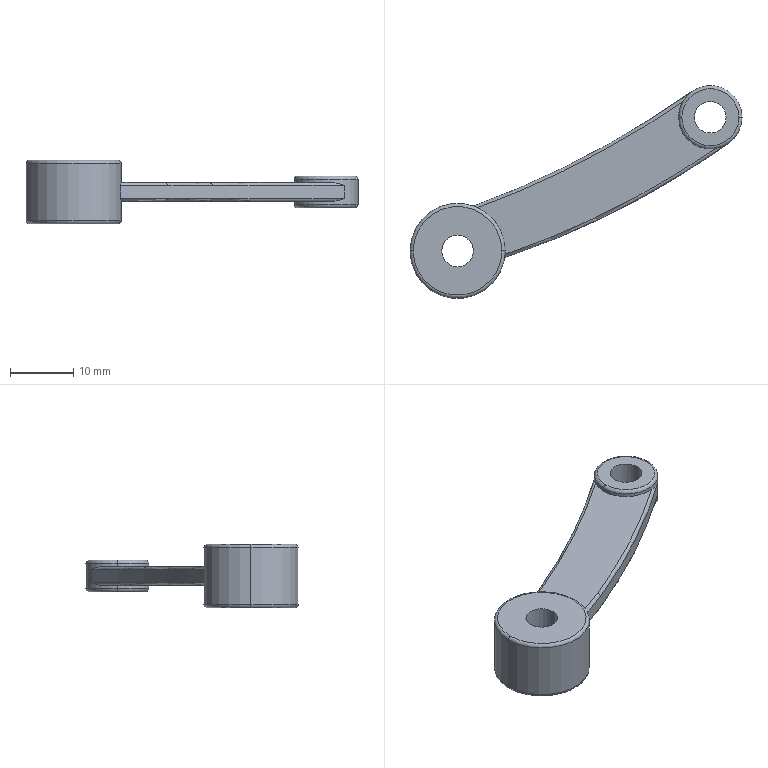Part | SolidWorks | features ICE 2, Extrusion 1, Fillet 1, MirrorPattern 1 | 1 solid | 28 faces | box 52.377 x 33.585 x 10 mm | volume 2859 mm3 | torus 12 | cylinder 10 | plane 6 | commonest cylinder face diameters 5 x4 10 x2 15 x2 270 x1 292 x1
STEP:
#1=CARTESIAN_POINT('',(-7.5,0.,4.5));
#2=VERTEX_POINT('',#1);
#3=CARTESIAN_POINT('',(7.5,0.,4.5));
#4=VERTEX_POINT('',#3);
#5=CARTESIAN_POINT('',(0.,0.,4.5));
#6=DIRECTION('',(0.,0.,-1.));
#7=DIRECTION('',(1.,0.,0.));
#8=AXIS2_PLACEMENT_3D('',#5,#6,#7);
#9=CIRCLE('',#8,7.5);
#10=EDGE_CURVE('',#2,#4,#9,.T.);
#11=ORIENTED_EDGE('',*,*,#10,.F.);
#12=CARTESIAN_POINT('',(-7.,0.,5.));
#13=VERTEX_POINT('',#12);
#14=CARTESIAN_POINT('',(-7.,0.,4.5));
#15=DIRECTION('',(0.,1.,0.));
#16=DIRECTION('',(-1.,0.,0.));
#17=AXIS2_PLACEMENT_3D('',#14,#15,#16);
#18=CIRCLE('',#17,0.5);
#19=EDGE_CURVE('',#2,#13,#18,.T.);
#20=ORIENTED_EDGE('',*,*,#19,.T.);
#21=CARTESIAN_POINT('',(7.,0.,5.));
#22=VERTEX_POINT('',#21);
#23=CARTESIAN_POINT('',(0.,0.,5.));
#24=DIRECTION('',(0.,0.,1.));
#25=DIRECTION('',(1.,0.,0.));
#26=AXIS2_PLACEMENT_3D('',#23,#24,#25);
#27=CIRCLE('',#26,7.);
#28=EDGE_CURVE('',#22,#13,#27,.T.);
#29=ORIENTED_EDGE('',*,*,#28,.F.);
#30=CARTESIAN_POINT('',(7.,0.,4.5));
#31=DIRECTION('',(0.,-1.,0.));
#32=DIRECTION('',(0.,0.,-1.));
#33=AXIS2_PLACEMENT_3D('',#30,#31,#32);
#34=CIRCLE('',#33,0.5);
#35=EDGE_CURVE('',#4,#22,#34,.T.);
#36=ORIENTED_EDGE('',*,*,#35,.F.);
#37=EDGE_LOOP('',(#11,#20,#29,#36));
#38=FACE_OUTER_BOUND('',#37,.T.);
#39=CARTESIAN_POINT('',(0.,0.,4.5));
#40=DIRECTION('',(0.,0.,1.));
#41=DIRECTION('',(1.,0.,0.));
#42=AXIS2_PLACEMENT_3D('',#39,#40,#41);
#43=TOROIDAL_SURFACE('',#42,7.,0.5);
#44=ADVANCED_FACE('',(#38),#43,.T.);
#45=CARTESIAN_POINT('',(-7.,0.,-5.));
#46=VERTEX_POINT('',#45);
#47=CARTESIAN_POINT('',(7.,0.,-5.));
#48=VERTEX_POINT('',#47);
#49=CARTESIAN_POINT('',(0.,0.,-5.));
#50=DIRECTION('',(0.,0.,-1.));
#51=DIRECTION('',(1.,0.,0.));
#52=AXIS2_PLACEMENT_3D('',#49,#50,#51);
#53=CIRCLE('',#52,7.);
#54=EDGE_CURVE('',#46,#48,#53,.T.);
#55=ORIENTED_EDGE('',*,*,#54,.F.);
#56=CARTESIAN_POINT('',(-7.5,0.,-4.5));
#57=VERTEX_POINT('',#56);
#58=CARTESIAN_POINT('',(-7.,0.,-4.5));
#59=DIRECTION('',(0.,1.,0.));
#60=DIRECTION('',(-1.,0.,0.));
#61=AXIS2_PLACEMENT_3D('',#58,#59,#60);
#62=CIRCLE('',#61,0.5);
#63=EDGE_CURVE('',#46,#57,#62,.T.);
#64=ORIENTED_EDGE('',*,*,#63,.T.);
#65=CARTESIAN_POINT('',(7.5,0.,-4.5));
#66=VERTEX_POINT('',#65);
#67=CARTESIAN_POINT('',(0.,0.,-4.5));
#68=DIRECTION('',(0.,0.,1.));
#69=DIRECTION('',(1.,0.,0.));
#70=AXIS2_PLACEMENT_3D('',#67,#68,#69);
#71=CIRCLE('',#70,7.5);
#72=EDGE_CURVE('',#66,#57,#71,.T.);
#73=ORIENTED_EDGE('',*,*,#72,.F.);
#74=CARTESIAN_POINT('',(7.,0.,-4.5));
#75=DIRECTION('',(0.,-1.,0.));
#76=DIRECTION('',(0.,0.,-1.));
#77=AXIS2_PLACEMENT_3D('',#74,#75,#76);
#78=CIRCLE('',#77,0.5);
#79=EDGE_CURVE('',#48,#66,#78,.T.);
#80=ORIENTED_EDGE('',*,*,#79,.F.);
#81=EDGE_LOOP('',(#55,#64,#73,#80));
#82=FACE_OUTER_BOUND('',#81,.T.);
#83=CARTESIAN_POINT('',(0.,0.,-4.5));
#84=DIRECTION('',(0.,0.,1.));
#85=DIRECTION('',(1.,0.,0.));
#86=AXIS2_PLACEMENT_3D('',#83,#84,#85);
#87=TOROIDAL_SURFACE('',#86,7.,0.5);
#88=ADVANCED_FACE('',(#82),#87,.T.);
#89=CARTESIAN_POINT('',(34.877,21.085,2.));
#90=VERTEX_POINT('',#89);
#91=CARTESIAN_POINT('',(44.877,21.085,2.));
#92=VERTEX_POINT('',#91);
#93=CARTESIAN_POINT('',(39.877,21.085,2.));
#94=DIRECTION('',(0.,0.,-1.));
#95=DIRECTION('',(1.,0.,0.));
#96=AXIS2_PLACEMENT_3D('',#93,#94,#95);
#97=CIRCLE('',#96,5.);
#98=EDGE_CURVE('',#90,#92,#97,.T.);
#99=ORIENTED_EDGE('',*,*,#98,.F.);
#100=CARTESIAN_POINT('',(35.377,21.085,2.5));
#101=VERTEX_POINT('',#100);
#102=CARTESIAN_POINT('',(35.377,21.085,2.));
#103=DIRECTION('',(0.,1.,0.));
#104=DIRECTION('',(-1.,0.,0.));
#105=AXIS2_PLACEMENT_3D('',#102,#103,#104);
#106=CIRCLE('',#105,0.5);
#107=EDGE_CURVE('',#90,#101,#106,.T.);
#108=ORIENTED_EDGE('',*,*,#107,.T.);
#109=CARTESIAN_POINT('',(44.377,21.085,2.5));
#110=VERTEX_POINT('',#109);
#111=CARTESIAN_POINT('',(39.877,21.085,2.5));
#112=DIRECTION('',(0.,0.,1.));
#113=DIRECTION('',(1.,0.,0.));
#114=AXIS2_PLACEMENT_3D('',#111,#112,#113);
#115=CIRCLE('',#114,4.5);
#116=EDGE_CURVE('',#110,#101,#115,.T.);
#117=ORIENTED_EDGE('',*,*,#116,.F.);
#118=CARTESIAN_POINT('',(44.377,21.085,2.));
#119=DIRECTION('',(0.,-1.,0.));
#120=DIRECTION('',(0.,0.,-1.));
#121=AXIS2_PLACEMENT_3D('',#118,#119,#120);
#122=CIRCLE('',#121,0.5);
#123=EDGE_CURVE('',#92,#110,#122,.T.);
#124=ORIENTED_EDGE('',*,*,#123,.F.);
#125=EDGE_LOOP('',(#99,#108,#117,#124));
#126=FACE_OUTER_BOUND('',#125,.T.);
#127=CARTESIAN_POINT('',(39.877,21.085,2.));
#128=DIRECTION('',(0.,0.,1.));
#129=DIRECTION('',(1.,0.,0.));
#130=AXIS2_PLACEMENT_3D('',#127,#128,#129);
#131=TOROIDAL_SURFACE('',#130,4.5,0.5);
#132=ADVANCED_FACE('',(#126),#131,.T.);
#133=CARTESIAN_POINT('',(44.877,21.085,-2.));
#134=VERTEX_POINT('',#133);
#135=CARTESIAN_POINT('',(34.877,21.085,-2.));
#136=VERTEX_POINT('',#135);
#137=CARTESIAN_POINT('',(39.877,21.085,-2.));
#138=DIRECTION('',(0.,0.,1.));
#139=DIRECTION('',(-1.,0.,0.));
#140=AXIS2_PLACEMENT_3D('',#137,#138,#139);
#141=CIRCLE('',#140,5.);
#142=EDGE_CURVE('',#134,#136,#141,.T.);
#143=ORIENTED_EDGE('',*,*,#142,.F.);
#144=CARTESIAN_POINT('',(44.377,21.085,-2.5));
#145=VERTEX_POINT('',#144);
#146=CARTESIAN_POINT('',(44.377,21.085,-2.));
#147=DIRECTION('',(0.,1.,0.));
#148=DIRECTION('',(-1.,0.,0.));
#149=AXIS2_PLACEMENT_3D('',#146,#147,#148);
#150=CIRCLE('',#149,0.5);
#151=EDGE_CURVE('',#134,#145,#150,.T.);
#152=ORIENTED_EDGE('',*,*,#151,.T.);
#153=CARTESIAN_POINT('',(35.377,21.085,-2.5));
#154=VERTEX_POINT('',#153);
#155=CARTESIAN_POINT('',(39.877,21.085,-2.5));
#156=DIRECTION('',(0.,0.,-1.));
#157=DIRECTION('',(-1.,0.,0.));
#158=AXIS2_PLACEMENT_3D('',#155,#156,#157);
#159=CIRCLE('',#158,4.5);
#160=EDGE_CURVE('',#154,#145,#159,.T.);
#161=ORIENTED_EDGE('',*,*,#160,.F.);
#162=CARTESIAN_POINT('',(35.377,21.085,-2.));
#163=DIRECTION('',(0.,-1.,0.));
#164=DIRECTION('',(0.,0.,-1.));
#165=AXIS2_PLACEMENT_3D('',#162,#163,#164);
#166=CIRCLE('',#165,0.5);
#167=EDGE_CURVE('',#136,#154,#166,.T.);
#168=ORIENTED_EDGE('',*,*,#167,.F.);
#169=EDGE_LOOP('',(#143,#152,#161,#168));
#170=FACE_OUTER_BOUND('',#169,.T.);
#171=CARTESIAN_POINT('',(39.877,21.085,-2.));
#172=DIRECTION('',(0.,0.,-1.));
#173=DIRECTION('',(-1.,0.,0.));
#174=AXIS2_PLACEMENT_3D('',#171,#172,#173);
#175=TOROIDAL_SURFACE('',#174,4.5,0.5);
#176=ADVANCED_FACE('',(#170),#175,.T.);
#177=CARTESIAN_POINT('',(37.377,21.085,2.5));
#178=VERTEX_POINT('',#177);
#179=CARTESIAN_POINT('',(42.377,21.085,2.5));
#180=VERTEX_POINT('',#179);
#181=CARTESIAN_POINT('',(39.877,21.085,2.5));
#182=DIRECTION('',(0.,0.,1.));
#183=DIRECTION('',(1.,0.,0.));
#184=AXIS2_PLACEMENT_3D('',#181,#182,#183);
#185=CIRCLE('',#184,2.5);
#186=EDGE_CURVE('',#178,#180,#185,.T.);
#187=ORIENTED_EDGE('',*,*,#186,.T.);
#188=CARTESIAN_POINT('',(42.377,21.085,-2.5));
#189=VERTEX_POINT('',#188);
#190=CARTESIAN_POINT('',(42.377,21.085,1.5));
#191=DIRECTION('',(0.,0.,-1.));
#192=VECTOR('',#191,1000.);
#193=LINE('',#190,#192);
#194=EDGE_CURVE('',#180,#189,#193,.T.);
#195=ORIENTED_EDGE('',*,*,#194,.T.);
#196=CARTESIAN_POINT('',(37.377,21.085,-2.5));
#197=VERTEX_POINT('',#196);
#198=CARTESIAN_POINT('',(39.877,21.085,-2.5));
#199=DIRECTION('',(0.,0.,1.));
#200=DIRECTION('',(1.,0.,0.));
#201=AXIS2_PLACEMENT_3D('',#198,#199,#200);
#202=CIRCLE('',#201,2.5);
#203=EDGE_CURVE('',#197,#189,#202,.T.);
#204=ORIENTED_EDGE('',*,*,#203,.F.);
#205=CARTESIAN_POINT('',(37.377,21.085,1.5));
#206=DIRECTION('',(0.,0.,-1.));
#207=VECTOR('',#206,1000.);
#208=LINE('',#205,#207);
#209=EDGE_CURVE('',#178,#197,#208,.T.);
#210=ORIENTED_EDGE('',*,*,#209,.F.);
#211=EDGE_LOOP('',(#187,#195,#204,#210));
#212=FACE_OUTER_BOUND('',#211,.T.);
#213=CARTESIAN_POINT('',(39.877,21.085,1.5));
#214=DIRECTION('',(0.,0.,-1.));
#215=DIRECTION('',(-1.,0.,0.));
#216=AXIS2_PLACEMENT_3D('',#213,#214,#215);
#217=CYLINDRICAL_SURFACE('',#216,2.5);
#218=ADVANCED_FACE('',(#212),#217,.F.);
#219=ORIENTED_EDGE('',*,*,#98,.T.);
#220=CARTESIAN_POINT('',(44.877,21.085,1.5));
#221=DIRECTION('',(0.,0.,-1.));
#222=VECTOR('',#221,1000.);
#223=LINE('',#220,#222);
#224=EDGE_CURVE('',#92,#134,#223,.T.);
#225=ORIENTED_EDGE('',*,*,#224,.T.);
#226=ORIENTED_EDGE('',*,*,#142,.T.);
#227=CARTESIAN_POINT('',(34.877,21.085,-1.5));
#228=VERTEX_POINT('',#227);
#229=CARTESIAN_POINT('',(34.877,21.085,1.5));
#230=DIRECTION('',(0.,0.,-1.));
#231=VECTOR('',#230,1000.);
#232=LINE('',#229,#231);
#233=EDGE_CURVE('',#228,#136,#232,.T.);
#234=ORIENTED_EDGE('',*,*,#233,.F.);
#235=CARTESIAN_POINT('',(35.515,23.53,-1.5));
#236=VERTEX_POINT('',#235);
#237=CARTESIAN_POINT('',(39.877,21.085,-1.5));
#238=DIRECTION('',(0.,0.,1.));
#239=DIRECTION('',(1.,0.,0.));
#240=AXIS2_PLACEMENT_3D('',#237,#238,#239);
#241=CIRCLE('',#240,5.);
#242=EDGE_CURVE('',#236,#228,#241,.T.);
#243=ORIENTED_EDGE('',*,*,#242,.F.);
#244=CARTESIAN_POINT('',(36.988,25.166,-1.));
#245=VERTEX_POINT('',#244);
#246=CARTESIAN_POINT('',(35.515,23.53,-1.5));
#247=CARTESIAN_POINT('',(35.609,23.698,-1.5));
#248=CARTESIAN_POINT('',(35.711,23.857,-1.479));
#249=CARTESIAN_POINT('',(35.93,24.161,-1.418));
#250=CARTESIAN_POINT('',(36.048,24.307,-1.376));
#251=CARTESIAN_POINT('',(36.296,24.58,-1.281));
#252=CARTESIAN_POINT('',(36.426,24.708,-1.228));
#253=CARTESIAN_POINT('',(36.697,24.948,-1.117));
#254=CARTESIAN_POINT('',(36.84,25.062,-1.058));
#255=CARTESIAN_POINT('',(36.988,25.166,-1.));
#256=B_SPLINE_CURVE_WITH_KNOTS('',3,(#246,#247,#248,#249,#250,#251,#252,#253,#254,#255),.UNSPECIFIED.,.F.,.F.,(4,2,2,2,4),(0.,0.0005692,0.001138,0.001708,0.002277),.UNSPECIFIED.);
#257=EDGE_CURVE('',#236,#245,#256,.T.);
#258=ORIENTED_EDGE('',*,*,#257,.T.);
#259=CARTESIAN_POINT('',(36.988,25.166,1.));
#260=VERTEX_POINT('',#259);
#261=CARTESIAN_POINT('',(36.988,25.166,1.5));
#262=DIRECTION('',(0.,0.,-1.));
#263=VECTOR('',#262,1000.);
#264=LINE('',#261,#263);
#265=EDGE_CURVE('',#260,#245,#264,.T.);
#266=ORIENTED_EDGE('',*,*,#265,.F.);
#267=CARTESIAN_POINT('',(35.515,23.53,1.5));
#268=VERTEX_POINT('',#267);
#269=CARTESIAN_POINT('',(36.988,25.166,1.));
#270=CARTESIAN_POINT('',(36.84,25.062,1.058));
#271=CARTESIAN_POINT('',(36.697,24.948,1.117));
#272=CARTESIAN_POINT('',(36.426,24.708,1.228));
#273=CARTESIAN_POINT('',(36.296,24.58,1.281));
#274=CARTESIAN_POINT('',(36.048,24.307,1.376));
#275=CARTESIAN_POINT('',(35.93,24.161,1.418));
#276=CARTESIAN_POINT('',(35.711,23.857,1.479));
#277=CARTESIAN_POINT('',(35.609,23.698,1.5));
#278=CARTESIAN_POINT('',(35.515,23.53,1.5));
#279=B_SPLINE_CURVE_WITH_KNOTS('',3,(#269,#270,#271,#272,#273,#274,#275,#276,#277,#278),.UNSPECIFIED.,.F.,.F.,(4,2,2,2,4),(-0.00001391,0.000555,0.001124,0.001693,0.002262),.UNSPECIFIED.);
#280=EDGE_CURVE('',#260,#268,#279,.T.);
#281=ORIENTED_EDGE('',*,*,#280,.T.);
#282=CARTESIAN_POINT('',(34.877,21.085,1.5));
#283=VERTEX_POINT('',#282);
#284=CARTESIAN_POINT('',(39.877,21.085,1.5));
#285=DIRECTION('',(0.,0.,1.));
#286=DIRECTION('',(1.,0.,0.));
#287=AXIS2_PLACEMENT_3D('',#284,#285,#286);
#288=CIRCLE('',#287,5.);
#289=EDGE_CURVE('',#268,#283,#288,.T.);
#290=ORIENTED_EDGE('',*,*,#289,.T.);
#291=CARTESIAN_POINT('',(34.877,21.085,1.5));
#292=DIRECTION('',(0.,0.,-1.));
#293=VECTOR('',#292,1000.);
#294=LINE('',#291,#293);
#295=EDGE_CURVE('',#90,#283,#294,.T.);
#296=ORIENTED_EDGE('',*,*,#295,.F.);
#297=EDGE_LOOP('',(#219,#225,#226,#234,#243,#258,#266,#281,#290,#296));
#298=FACE_OUTER_BOUND('',#297,.T.);
#299=CARTESIAN_POINT('',(39.877,21.085,1.5));
#300=DIRECTION('',(0.,0.,-1.));
#301=DIRECTION('',(-1.,0.,0.));
#302=AXIS2_PLACEMENT_3D('',#299,#300,#301);
#303=CYLINDRICAL_SURFACE('',#302,5.);
#304=ADVANCED_FACE('',(#298),#303,.T.);
#305=CARTESIAN_POINT('',(-2.5,0.,5.));
#306=VERTEX_POINT('',#305);
#307=CARTESIAN_POINT('',(2.5,0.,5.));
#308=VERTEX_POINT('',#307);
#309=CARTESIAN_POINT('',(0.,0.,5.));
#310=DIRECTION('',(0.,0.,1.));
#311=DIRECTION('',(1.,0.,0.));
#312=AXIS2_PLACEMENT_3D('',#309,#310,#311);
#313=CIRCLE('',#312,2.5);
#314=EDGE_CURVE('',#306,#308,#313,.T.);
#315=ORIENTED_EDGE('',*,*,#314,.T.);
#316=CARTESIAN_POINT('',(2.5,0.,-5.));
#317=VERTEX_POINT('',#316);
#318=CARTESIAN_POINT('',(2.5,0.,5.));
#319=DIRECTION('',(0.,0.,-1.));
#320=VECTOR('',#319,1000.);
#321=LINE('',#318,#320);
#322=EDGE_CURVE('',#308,#317,#321,.T.);
#323=ORIENTED_EDGE('',*,*,#322,.T.);
#324=CARTESIAN_POINT('',(-2.5,0.,-5.));
#325=VERTEX_POINT('',#324);
#326=CARTESIAN_POINT('',(0.,0.,-5.));
#327=DIRECTION('',(0.,0.,1.));
#328=DIRECTION('',(1.,0.,0.));
#329=AXIS2_PLACEMENT_3D('',#326,#327,#328);
#330=CIRCLE('',#329,2.5);
#331=EDGE_CURVE('',#325,#317,#330,.T.);
#332=ORIENTED_EDGE('',*,*,#331,.F.);
#333=CARTESIAN_POINT('',(-2.5,0.,5.));
#334=DIRECTION('',(0.,0.,-1.));
#335=VECTOR('',#334,1000.);
#336=LINE('',#333,#335);
#337=EDGE_CURVE('',#306,#325,#336,.T.);
#338=ORIENTED_EDGE('',*,*,#337,.F.);
#339=EDGE_LOOP('',(#315,#323,#332,#338));
#340=FACE_OUTER_BOUND('',#339,.T.);
#341=CARTESIAN_POINT('',(0.,0.,5.));
#342=DIRECTION('',(0.,0.,-1.));
#343=DIRECTION('',(-1.,0.,0.));
#344=AXIS2_PLACEMENT_3D('',#341,#342,#343);
#345=CYLINDRICAL_SURFACE('',#344,2.5);
#346=ADVANCED_FACE('',(#340),#345,.F.);
#347=ORIENTED_EDGE('',*,*,#10,.T.);
#348=CARTESIAN_POINT('',(7.5,0.,1.5));
#349=VERTEX_POINT('',#348);
#350=CARTESIAN_POINT('',(7.5,0.,5.));
#351=DIRECTION('',(0.,0.,-1.));
#352=VECTOR('',#351,1000.);
#353=LINE('',#350,#352);
#354=EDGE_CURVE('',#4,#349,#353,.T.);
#355=ORIENTED_EDGE('',*,*,#354,.T.);
#356=CARTESIAN_POINT('',(3.138,6.812,1.5));
#357=VERTEX_POINT('',#356);
#358=CARTESIAN_POINT('',(0.,0.,1.5));
#359=DIRECTION('',(0.,0.,-1.));
#360=DIRECTION('',(-1.,0.,0.));
#361=AXIS2_PLACEMENT_3D('',#358,#359,#360);
#362=CIRCLE('',#361,7.5);
#363=EDGE_CURVE('',#357,#349,#362,.T.);
#364=ORIENTED_EDGE('',*,*,#363,.F.);
#365=CARTESIAN_POINT('',(2.444,7.091,1.));
#366=VERTEX_POINT('',#365);
#367=CARTESIAN_POINT('',(3.138,6.812,1.5));
#368=CARTESIAN_POINT('',(3.063,6.847,1.5));
#369=CARTESIAN_POINT('',(2.989,6.879,1.49));
#370=CARTESIAN_POINT('',(2.843,6.941,1.451));
#371=CARTESIAN_POINT('',(2.77,6.97,1.422));
#372=CARTESIAN_POINT('',(2.637,7.022,1.343));
#373=CARTESIAN_POINT('',(2.574,7.045,1.292));
#374=CARTESIAN_POINT('',(2.477,7.079,1.163));
#375=CARTESIAN_POINT('',(2.444,7.091,1.083));
#376=CARTESIAN_POINT('',(2.444,7.091,1.));
#377=B_SPLINE_CURVE_WITH_KNOTS('',3,(#367,#368,#369,#370,#371,#372,#373,#374,#375,#376),.UNSPECIFIED.,.F.,.F.,(4,2,2,2,4),(0.,0.0002444,0.0004888,0.0007333,0.0009777),.UNSPECIFIED.);
#378=EDGE_CURVE('',#357,#366,#377,.T.);
#379=ORIENTED_EDGE('',*,*,#378,.T.);
#380=CARTESIAN_POINT('',(2.444,7.091,-1.));
#381=VERTEX_POINT('',#380);
#382=CARTESIAN_POINT('',(2.444,7.091,1.5));
#383=DIRECTION('',(0.,0.,-1.));
#384=VECTOR('',#383,1000.);
#385=LINE('',#382,#384);
#386=EDGE_CURVE('',#366,#381,#385,.T.);
#387=ORIENTED_EDGE('',*,*,#386,.T.);
#388=CARTESIAN_POINT('',(3.138,6.812,-1.5));
#389=VERTEX_POINT('',#388);
#390=CARTESIAN_POINT('',(2.444,7.091,-1.));
#391=CARTESIAN_POINT('',(2.444,7.091,-1.083));
#392=CARTESIAN_POINT('',(2.476,7.08,-1.162));
#393=CARTESIAN_POINT('',(2.574,7.045,-1.292));
#394=CARTESIAN_POINT('',(2.636,7.022,-1.342));
#395=CARTESIAN_POINT('',(2.837,6.944,-1.462));
#396=CARTESIAN_POINT('',(2.988,6.881,-1.5));
#397=CARTESIAN_POINT('',(3.138,6.812,-1.5));
#398=B_SPLINE_CURVE_WITH_KNOTS('',3,(#390,#391,#392,#393,#394,#395,#396,#397),.UNSPECIFIED.,.F.,.F.,(4,2,2,4),(0.,0.0002455,0.0004911,0.0009821),.UNSPECIFIED.);
#399=EDGE_CURVE('',#381,#389,#398,.T.);
#400=ORIENTED_EDGE('',*,*,#399,.T.);
#401=CARTESIAN_POINT('',(7.5,0.,-1.5));
#402=VERTEX_POINT('',#401);
#403=CARTESIAN_POINT('',(0.,0.,-1.5));
#404=DIRECTION('',(0.,0.,-1.));
#405=DIRECTION('',(-1.,0.,0.));
#406=AXIS2_PLACEMENT_3D('',#403,#404,#405);
#407=CIRCLE('',#406,7.5);
#408=EDGE_CURVE('',#389,#402,#407,.T.);
#409=ORIENTED_EDGE('',*,*,#408,.T.);
#410=CARTESIAN_POINT('',(7.5,0.,5.));
#411=DIRECTION('',(0.,0.,-1.));
#412=VECTOR('',#411,1000.);
#413=LINE('',#410,#412);
#414=EDGE_CURVE('',#402,#66,#413,.T.);
#415=ORIENTED_EDGE('',*,*,#414,.T.);
#416=ORIENTED_EDGE('',*,*,#72,.T.);
#417=CARTESIAN_POINT('',(-7.5,0.,5.));
#418=DIRECTION('',(0.,0.,-1.));
#419=VECTOR('',#418,1000.);
#420=LINE('',#417,#419);
#421=EDGE_CURVE('',#2,#57,#420,.T.);
#422=ORIENTED_EDGE('',*,*,#421,.F.);
#423=EDGE_LOOP('',(#347,#355,#364,#379,#387,#400,#409,#415,#416,#422));
#424=FACE_OUTER_BOUND('',#423,.T.);
#425=CARTESIAN_POINT('',(0.,0.,5.));
#426=DIRECTION('',(0.,0.,-1.));
#427=DIRECTION('',(-1.,0.,0.));
#428=AXIS2_PLACEMENT_3D('',#425,#426,#427);
#429=CYLINDRICAL_SURFACE('',#428,7.5);
#430=ADVANCED_FACE('',(#424),#429,.T.);
#431=ORIENTED_EDGE('',*,*,#289,.F.);
#432=CARTESIAN_POINT('',(-47.367,144.331,1.5));
#433=DIRECTION('',(0.,0.,-1.));
#434=DIRECTION('',(1.,0.,0.));
#435=AXIS2_PLACEMENT_3D('',#432,#433,#434);
#436=CIRCLE('',#435,146.5);
#437=EDGE_CURVE('',#268,#357,#436,.T.);
#438=ORIENTED_EDGE('',*,*,#437,.T.);
#439=ORIENTED_EDGE('',*,*,#363,.T.);
#440=CARTESIAN_POINT('',(7.482,-0.5227,1.5));
#441=VERTEX_POINT('',#440);
#442=CARTESIAN_POINT('',(0.,0.,1.5));
#443=DIRECTION('',(0.,0.,-1.));
#444=DIRECTION('',(-1.,0.,0.));
#445=AXIS2_PLACEMENT_3D('',#442,#443,#444);
#446=CIRCLE('',#445,7.5);
#447=EDGE_CURVE('',#349,#441,#446,.T.);
#448=ORIENTED_EDGE('',*,*,#447,.T.);
#449=CARTESIAN_POINT('',(40.679,16.15,1.5));
#450=VERTEX_POINT('',#449);
#451=CARTESIAN_POINT('',(-35.706,126.855,1.5));
#452=DIRECTION('',(0.,0.,1.));
#453=DIRECTION('',(1.,0.,0.));
#454=AXIS2_PLACEMENT_3D('',#451,#452,#453);
#455=CIRCLE('',#454,134.5);
#456=EDGE_CURVE('',#441,#450,#455,.T.);
#457=ORIENTED_EDGE('',*,*,#456,.T.);
#458=CARTESIAN_POINT('',(39.877,21.085,1.5));
#459=DIRECTION('',(0.,0.,1.));
#460=DIRECTION('',(1.,0.,0.));
#461=AXIS2_PLACEMENT_3D('',#458,#459,#460);
#462=CIRCLE('',#461,5.);
#463=EDGE_CURVE('',#283,#450,#462,.T.);
#464=ORIENTED_EDGE('',*,*,#463,.F.);
#465=EDGE_LOOP('',(#431,#438,#439,#448,#457,#464));
#466=FACE_OUTER_BOUND('',#465,.T.);
#467=CARTESIAN_POINT('',(2.085,73.97,1.5));
#468=DIRECTION('',(0.,0.,1.));
#469=DIRECTION('',(1.,0.,0.));
#470=AXIS2_PLACEMENT_3D('',#467,#468,#469);
#471=PLANE('',#470);
#472=ADVANCED_FACE('',(#466),#471,.T.);
#473=ORIENTED_EDGE('',*,*,#354,.F.);
#474=CARTESIAN_POINT('',(0.,0.,4.5));
#475=DIRECTION('',(0.,0.,-1.));
#476=DIRECTION('',(1.,0.,0.));
#477=AXIS2_PLACEMENT_3D('',#474,#475,#476);
#478=CIRCLE('',#477,7.5);
#479=EDGE_CURVE('',#4,#2,#478,.T.);
#480=ORIENTED_EDGE('',*,*,#479,.T.);
#481=ORIENTED_EDGE('',*,*,#421,.T.);
#482=CARTESIAN_POINT('',(0.,0.,-4.5));
#483=DIRECTION('',(0.,0.,1.));
#484=DIRECTION('',(1.,0.,0.));
#485=AXIS2_PLACEMENT_3D('',#482,#483,#484);
#486=CIRCLE('',#485,7.5);
#487=EDGE_CURVE('',#57,#66,#486,.T.);
#488=ORIENTED_EDGE('',*,*,#487,.T.);
#489=ORIENTED_EDGE('',*,*,#414,.F.);
#490=CARTESIAN_POINT('',(7.482,-0.5227,-1.5));
#491=VERTEX_POINT('',#490);
#492=CARTESIAN_POINT('',(0.,0.,-1.5));
#493=DIRECTION('',(0.,0.,-1.));
#494=DIRECTION('',(-1.,0.,0.));
#495=AXIS2_PLACEMENT_3D('',#492,#493,#494);
#496=CIRCLE('',#495,7.5);
#497=EDGE_CURVE('',#402,#491,#496,.T.);
#498=ORIENTED_EDGE('',*,*,#497,.T.);
#499=CARTESIAN_POINT('',(7.423,-1.07,-1.));
#500=VERTEX_POINT('',#499);
#501=CARTESIAN_POINT('',(7.482,-0.5227,-1.5));
#502=CARTESIAN_POINT('',(7.472,-0.6611,-1.5));
#503=CARTESIAN_POINT('',(7.458,-0.7962,-1.451));
#504=CARTESIAN_POINT('',(7.433,-1.004,-1.271));
#505=CARTESIAN_POINT('',(7.423,-1.07,-1.139));
#506=CARTESIAN_POINT('',(7.423,-1.07,-1.));
#507=B_SPLINE_CURVE_WITH_KNOTS('',3,(#501,#502,#503,#504,#505,#506),.UNSPECIFIED.,.F.,.F.,(4,2,4),(0.,0.0004102,0.0008204),.UNSPECIFIED.);
#508=EDGE_CURVE('',#491,#500,#507,.T.);
#509=ORIENTED_EDGE('',*,*,#508,.T.);
#510=CARTESIAN_POINT('',(7.423,-1.07,1.));
#511=VERTEX_POINT('',#510);
#512=CARTESIAN_POINT('',(7.423,-1.07,1.5));
#513=DIRECTION('',(0.,0.,-1.));
#514=VECTOR('',#513,1000.);
#515=LINE('',#512,#514);
#516=EDGE_CURVE('',#511,#500,#515,.T.);
#517=ORIENTED_EDGE('',*,*,#516,.F.);
#518=CARTESIAN_POINT('',(7.423,-1.07,1.));
#519=CARTESIAN_POINT('',(7.423,-1.07,1.139));
#520=CARTESIAN_POINT('',(7.433,-1.003,1.271));
#521=CARTESIAN_POINT('',(7.458,-0.7972,1.451));
#522=CARTESIAN_POINT('',(7.472,-0.6609,1.5));
#523=CARTESIAN_POINT('',(7.482,-0.5227,1.5));
#524=B_SPLINE_CURVE_WITH_KNOTS('',3,(#518,#519,#520,#521,#522,#523),.UNSPECIFIED.,.F.,.F.,(4,2,4),(0.,0.0004102,0.0008203),.UNSPECIFIED.);
#525=EDGE_CURVE('',#511,#441,#524,.T.);
#526=ORIENTED_EDGE('',*,*,#525,.T.);
#527=ORIENTED_EDGE('',*,*,#447,.F.);
#528=EDGE_LOOP('',(#473,#480,#481,#488,#489,#498,#509,#517,#526,#527));
#529=FACE_OUTER_BOUND('',#528,.T.);
#530=CARTESIAN_POINT('',(0.,0.,5.));
#531=DIRECTION('',(0.,0.,-1.));
#532=DIRECTION('',(-1.,0.,0.));
#533=AXIS2_PLACEMENT_3D('',#530,#531,#532);
#534=CYLINDRICAL_SURFACE('',#533,7.5);
#535=ADVANCED_FACE('',(#529),#534,.T.);
#536=ORIENTED_EDGE('',*,*,#28,.T.);
#537=CARTESIAN_POINT('',(0.,0.,5.));
#538=DIRECTION('',(0.,0.,1.));
#539=DIRECTION('',(1.,0.,0.));
#540=AXIS2_PLACEMENT_3D('',#537,#538,#539);
#541=CIRCLE('',#540,7.);
#542=EDGE_CURVE('',#13,#22,#541,.T.);
#543=ORIENTED_EDGE('',*,*,#542,.T.);
#544=EDGE_LOOP('',(#536,#543));
#545=FACE_OUTER_BOUND('',#544,.T.);
#546=ORIENTED_EDGE('',*,*,#314,.F.);
#547=CARTESIAN_POINT('',(0.,0.,5.));
#548=DIRECTION('',(0.,0.,1.));
#549=DIRECTION('',(1.,0.,0.));
#550=AXIS2_PLACEMENT_3D('',#547,#548,#549);
#551=CIRCLE('',#550,2.5);
#552=EDGE_CURVE('',#308,#306,#551,.T.);
#553=ORIENTED_EDGE('',*,*,#552,.F.);
#554=EDGE_LOOP('',(#546,#553));
#555=FACE_BOUND('',#554,.T.);
#556=CARTESIAN_POINT('',(0.,0.,5.));
#557=DIRECTION('',(0.,0.,1.));
#558=DIRECTION('',(1.,0.,0.));
#559=AXIS2_PLACEMENT_3D('',#556,#557,#558);
#560=PLANE('',#559);
#561=ADVANCED_FACE('',(#545,#555),#560,.T.);
#562=CARTESIAN_POINT('',(0.,0.,-5.));
#563=DIRECTION('',(0.,0.,-1.));
#564=DIRECTION('',(1.,0.,0.));
#565=AXIS2_PLACEMENT_3D('',#562,#563,#564);
#566=CIRCLE('',#565,7.);
#567=EDGE_CURVE('',#48,#46,#566,.T.);
#568=ORIENTED_EDGE('',*,*,#567,.T.);
#569=ORIENTED_EDGE('',*,*,#54,.T.);
#570=EDGE_LOOP('',(#568,#569));
#571=FACE_OUTER_BOUND('',#570,.T.);
#572=ORIENTED_EDGE('',*,*,#331,.T.);
#573=CARTESIAN_POINT('',(0.,0.,-5.));
#574=DIRECTION('',(0.,0.,1.));
#575=DIRECTION('',(1.,0.,0.));
#576=AXIS2_PLACEMENT_3D('',#573,#574,#575);
#577=CIRCLE('',#576,2.5);
#578=EDGE_CURVE('',#317,#325,#577,.T.);
#579=ORIENTED_EDGE('',*,*,#578,.T.);
#580=EDGE_LOOP('',(#572,#579));
#581=FACE_BOUND('',#580,.T.);
#582=CARTESIAN_POINT('',(0.,0.,-5.));
#583=DIRECTION('',(0.,0.,1.));
#584=DIRECTION('',(1.,0.,0.));
#585=AXIS2_PLACEMENT_3D('',#582,#583,#584);
#586=PLANE('',#585);
#587=ADVANCED_FACE('',(#571,#581),#586,.F.);
#588=ORIENTED_EDGE('',*,*,#322,.F.);
#589=ORIENTED_EDGE('',*,*,#552,.T.);
#590=ORIENTED_EDGE('',*,*,#337,.T.);
#591=ORIENTED_EDGE('',*,*,#578,.F.);
#592=EDGE_LOOP('',(#588,#589,#590,#591));
#593=FACE_OUTER_BOUND('',#592,.T.);
#594=CARTESIAN_POINT('',(0.,0.,5.));
#595=DIRECTION('',(0.,0.,-1.));
#596=DIRECTION('',(-1.,0.,0.));
#597=AXIS2_PLACEMENT_3D('',#594,#595,#596);
#598=CYLINDRICAL_SURFACE('',#597,2.5);
#599=ADVANCED_FACE('',(#593),#598,.F.);
#600=ORIENTED_EDGE('',*,*,#408,.F.);
#601=CARTESIAN_POINT('',(-47.367,144.331,-1.5));
#602=DIRECTION('',(0.,0.,1.));
#603=DIRECTION('',(1.,0.,0.));
#604=AXIS2_PLACEMENT_3D('',#601,#602,#603);
#605=CIRCLE('',#604,146.5);
#606=EDGE_CURVE('',#389,#236,#605,.T.);
#607=ORIENTED_EDGE('',*,*,#606,.T.);
#608=ORIENTED_EDGE('',*,*,#242,.T.);
#609=CARTESIAN_POINT('',(40.679,16.15,-1.5));
#610=VERTEX_POINT('',#609);
#611=CARTESIAN_POINT('',(39.877,21.085,-1.5));
#612=DIRECTION('',(0.,0.,1.));
#613=DIRECTION('',(1.,0.,0.));
#614=AXIS2_PLACEMENT_3D('',#611,#612,#613);
#615=CIRCLE('',#614,5.);
#616=EDGE_CURVE('',#228,#610,#615,.T.);
#617=ORIENTED_EDGE('',*,*,#616,.T.);
#618=CARTESIAN_POINT('',(-35.706,126.855,-1.5));
#619=DIRECTION('',(0.,0.,-1.));
#620=DIRECTION('',(1.,0.,0.));
#621=AXIS2_PLACEMENT_3D('',#618,#619,#620);
#622=CIRCLE('',#621,134.5);
#623=EDGE_CURVE('',#610,#491,#622,.T.);
#624=ORIENTED_EDGE('',*,*,#623,.T.);
#625=ORIENTED_EDGE('',*,*,#497,.F.);
#626=EDGE_LOOP('',(#600,#607,#608,#617,#624,#625));
#627=FACE_OUTER_BOUND('',#626,.T.);
#628=CARTESIAN_POINT('',(2.085,73.97,-1.5));
#629=DIRECTION('',(0.,0.,1.));
#630=DIRECTION('',(1.,0.,0.));
#631=AXIS2_PLACEMENT_3D('',#628,#629,#630);
#632=PLANE('',#631);
#633=ADVANCED_FACE('',(#627),#632,.F.);
#634=ORIENTED_EDGE('',*,*,#516,.T.);
#635=CARTESIAN_POINT('',(42.784,17.017,-1.));
#636=VERTEX_POINT('',#635);
#637=CARTESIAN_POINT('',(-35.706,126.855,-1.));
#638=DIRECTION('',(0.,0.,1.));
#639=DIRECTION('',(1.,0.,0.));
#640=AXIS2_PLACEMENT_3D('',#637,#638,#639);
#641=CIRCLE('',#640,135.);
#642=EDGE_CURVE('',#500,#636,#641,.T.);
#643=ORIENTED_EDGE('',*,*,#642,.T.);
#644=CARTESIAN_POINT('',(42.784,17.017,1.));
#645=VERTEX_POINT('',#644);
#646=CARTESIAN_POINT('',(42.784,17.017,1.5));
#647=DIRECTION('',(0.,0.,-1.));
#648=VECTOR('',#647,1000.);
#649=LINE('',#646,#648);
#650=EDGE_CURVE('',#645,#636,#649,.T.);
#651=ORIENTED_EDGE('',*,*,#650,.F.);
#652=CARTESIAN_POINT('',(-35.706,126.855,1.));
#653=DIRECTION('',(0.,0.,-1.));
#654=DIRECTION('',(1.,0.,0.));
#655=AXIS2_PLACEMENT_3D('',#652,#653,#654);
#656=CIRCLE('',#655,135.);
#657=EDGE_CURVE('',#645,#511,#656,.T.);
#658=ORIENTED_EDGE('',*,*,#657,.T.);
#659=EDGE_LOOP('',(#634,#643,#651,#658));
#660=FACE_OUTER_BOUND('',#659,.T.);
#661=CARTESIAN_POINT('',(-35.706,126.855,1.5));
#662=DIRECTION('',(0.,0.,-1.));
#663=DIRECTION('',(-1.,0.,0.));
#664=AXIS2_PLACEMENT_3D('',#661,#662,#663);
#665=CYLINDRICAL_SURFACE('',#664,135.);
#666=ADVANCED_FACE('',(#660),#665,.T.);
#667=ORIENTED_EDGE('',*,*,#224,.F.);
#668=CARTESIAN_POINT('',(39.877,21.085,2.));
#669=DIRECTION('',(0.,0.,-1.));
#670=DIRECTION('',(1.,0.,0.));
#671=AXIS2_PLACEMENT_3D('',#668,#669,#670);
#672=CIRCLE('',#671,5.);
#673=EDGE_CURVE('',#92,#90,#672,.T.);
#674=ORIENTED_EDGE('',*,*,#673,.T.);
#675=ORIENTED_EDGE('',*,*,#295,.T.);
#676=ORIENTED_EDGE('',*,*,#463,.T.);
#677=CARTESIAN_POINT('',(40.679,16.15,1.5));
#678=CARTESIAN_POINT('',(40.875,16.182,1.5));
#679=CARTESIAN_POINT('',(41.065,16.224,1.479));
#680=CARTESIAN_POINT('',(41.438,16.331,1.418));
#681=CARTESIAN_POINT('',(41.621,16.395,1.376));
#682=CARTESIAN_POINT('',(41.973,16.542,1.281));
#683=CARTESIAN_POINT('',(42.143,16.624,1.228));
#684=CARTESIAN_POINT('',(42.471,16.807,1.117));
#685=CARTESIAN_POINT('',(42.631,16.908,1.058));
#686=CARTESIAN_POINT('',(42.784,17.017,1.));
#687=B_SPLINE_CURVE_WITH_KNOTS('',3,(#677,#678,#679,#680,#681,#682,#683,#684,#685,#686),.UNSPECIFIED.,.F.,.F.,(4,2,2,2,4),(0.,0.0005882,0.001176,0.001765,0.002353),.UNSPECIFIED.);
#688=EDGE_CURVE('',#450,#645,#687,.T.);
#689=ORIENTED_EDGE('',*,*,#688,.T.);
#690=ORIENTED_EDGE('',*,*,#650,.T.);
#691=CARTESIAN_POINT('',(42.784,17.017,-1.));
#692=CARTESIAN_POINT('',(42.631,16.908,-1.058));
#693=CARTESIAN_POINT('',(42.471,16.807,-1.117));
#694=CARTESIAN_POINT('',(42.143,16.624,-1.228));
#695=CARTESIAN_POINT('',(41.973,16.542,-1.281));
#696=CARTESIAN_POINT('',(41.621,16.395,-1.376));
#697=CARTESIAN_POINT('',(41.438,16.331,-1.418));
#698=CARTESIAN_POINT('',(41.065,16.224,-1.479));
#699=CARTESIAN_POINT('',(40.875,16.182,-1.5));
#700=CARTESIAN_POINT('',(40.679,16.15,-1.5));
#701=B_SPLINE_CURVE_WITH_KNOTS('',3,(#691,#692,#693,#694,#695,#696,#697,#698,#699,#700),.UNSPECIFIED.,.F.,.F.,(4,2,2,2,4),(-0.00001441,0.0005732,0.001161,0.001749,0.002336),.UNSPECIFIED.);
#702=EDGE_CURVE('',#636,#610,#701,.T.);
#703=ORIENTED_EDGE('',*,*,#702,.T.);
#704=ORIENTED_EDGE('',*,*,#616,.F.);
#705=ORIENTED_EDGE('',*,*,#233,.T.);
#706=CARTESIAN_POINT('',(39.877,21.085,-2.));
#707=DIRECTION('',(0.,0.,1.));
#708=DIRECTION('',(-1.,0.,0.));
#709=AXIS2_PLACEMENT_3D('',#706,#707,#708);
#710=CIRCLE('',#709,5.);
#711=EDGE_CURVE('',#136,#134,#710,.T.);
#712=ORIENTED_EDGE('',*,*,#711,.T.);
#713=EDGE_LOOP('',(#667,#674,#675,#676,#689,#690,#703,#704,#705,#712));
#714=FACE_OUTER_BOUND('',#713,.T.);
#715=CARTESIAN_POINT('',(39.877,21.085,1.5));
#716=DIRECTION('',(0.,0.,-1.));
#717=DIRECTION('',(-1.,0.,0.));
#718=AXIS2_PLACEMENT_3D('',#715,#716,#717);
#719=CYLINDRICAL_SURFACE('',#718,5.);
#720=ADVANCED_FACE('',(#714),#719,.T.);
#721=ORIENTED_EDGE('',*,*,#265,.T.);
#722=CARTESIAN_POINT('',(-47.367,144.331,-1.));
#723=DIRECTION('',(0.,0.,-1.));
#724=DIRECTION('',(1.,0.,0.));
#725=AXIS2_PLACEMENT_3D('',#722,#723,#724);
#726=CIRCLE('',#725,146.);
#727=EDGE_CURVE('',#245,#381,#726,.T.);
#728=ORIENTED_EDGE('',*,*,#727,.T.);
#729=ORIENTED_EDGE('',*,*,#386,.F.);
#730=CARTESIAN_POINT('',(-47.367,144.331,1.));
#731=DIRECTION('',(0.,0.,1.));
#732=DIRECTION('',(1.,0.,0.));
#733=AXIS2_PLACEMENT_3D('',#730,#731,#732);
#734=CIRCLE('',#733,146.);
#735=EDGE_CURVE('',#366,#260,#734,.T.);
#736=ORIENTED_EDGE('',*,*,#735,.T.);
#737=EDGE_LOOP('',(#721,#728,#729,#736));
#738=FACE_OUTER_BOUND('',#737,.T.);
#739=CARTESIAN_POINT('',(-47.367,144.331,1.5));
#740=DIRECTION('',(0.,0.,-1.));
#741=DIRECTION('',(-1.,0.,0.));
#742=AXIS2_PLACEMENT_3D('',#739,#740,#741);
#743=CYLINDRICAL_SURFACE('',#742,146.);
#744=ADVANCED_FACE('',(#738),#743,.F.);
#745=ORIENTED_EDGE('',*,*,#194,.F.);
#746=CARTESIAN_POINT('',(39.877,21.085,2.5));
#747=DIRECTION('',(0.,0.,1.));
#748=DIRECTION('',(1.,0.,0.));
#749=AXIS2_PLACEMENT_3D('',#746,#747,#748);
#750=CIRCLE('',#749,2.5);
#751=EDGE_CURVE('',#180,#178,#750,.T.);
#752=ORIENTED_EDGE('',*,*,#751,.T.);
#753=ORIENTED_EDGE('',*,*,#209,.T.);
#754=CARTESIAN_POINT('',(39.877,21.085,-2.5));
#755=DIRECTION('',(0.,0.,1.));
#756=DIRECTION('',(1.,0.,0.));
#757=AXIS2_PLACEMENT_3D('',#754,#755,#756);
#758=CIRCLE('',#757,2.5);
#759=EDGE_CURVE('',#189,#197,#758,.T.);
#760=ORIENTED_EDGE('',*,*,#759,.F.);
#761=EDGE_LOOP('',(#745,#752,#753,#760));
#762=FACE_OUTER_BOUND('',#761,.T.);
#763=CARTESIAN_POINT('',(39.877,21.085,1.5));
#764=DIRECTION('',(0.,0.,-1.));
#765=DIRECTION('',(-1.,0.,0.));
#766=AXIS2_PLACEMENT_3D('',#763,#764,#765);
#767=CYLINDRICAL_SURFACE('',#766,2.5);
#768=ADVANCED_FACE('',(#762),#767,.F.);
#769=ORIENTED_EDGE('',*,*,#116,.T.);
#770=CARTESIAN_POINT('',(39.877,21.085,2.5));
#771=DIRECTION('',(0.,0.,1.));
#772=DIRECTION('',(1.,0.,0.));
#773=AXIS2_PLACEMENT_3D('',#770,#771,#772);
#774=CIRCLE('',#773,4.5);
#775=EDGE_CURVE('',#101,#110,#774,.T.);
#776=ORIENTED_EDGE('',*,*,#775,.T.);
#777=EDGE_LOOP('',(#769,#776));
#778=FACE_OUTER_BOUND('',#777,.T.);
#779=ORIENTED_EDGE('',*,*,#186,.F.);
#780=ORIENTED_EDGE('',*,*,#751,.F.);
#781=EDGE_LOOP('',(#779,#780));
#782=FACE_BOUND('',#781,.T.);
#783=CARTESIAN_POINT('',(39.877,21.085,2.5));
#784=DIRECTION('',(0.,0.,1.));
#785=DIRECTION('',(1.,0.,0.));
#786=AXIS2_PLACEMENT_3D('',#783,#784,#785);
#787=PLANE('',#786);
#788=ADVANCED_FACE('',(#778,#782),#787,.T.);
#789=ORIENTED_EDGE('',*,*,#160,.T.);
#790=CARTESIAN_POINT('',(39.877,21.085,-2.5));
#791=DIRECTION('',(0.,0.,-1.));
#792=DIRECTION('',(-1.,0.,0.));
#793=AXIS2_PLACEMENT_3D('',#790,#791,#792);
#794=CIRCLE('',#793,4.5);
#795=EDGE_CURVE('',#145,#154,#794,.T.);
#796=ORIENTED_EDGE('',*,*,#795,.T.);
#797=EDGE_LOOP('',(#789,#796));
#798=FACE_OUTER_BOUND('',#797,.T.);
#799=ORIENTED_EDGE('',*,*,#203,.T.);
#800=ORIENTED_EDGE('',*,*,#759,.T.);
#801=EDGE_LOOP('',(#799,#800));
#802=FACE_BOUND('',#801,.T.);
#803=CARTESIAN_POINT('',(39.877,21.085,-2.5));
#804=DIRECTION('',(0.,0.,-1.));
#805=DIRECTION('',(1.,0.,0.));
#806=AXIS2_PLACEMENT_3D('',#803,#804,#805);
#807=PLANE('',#806);
#808=ADVANCED_FACE('',(#798,#802),#807,.T.);
#809=ORIENTED_EDGE('',*,*,#257,.F.);
#810=ORIENTED_EDGE('',*,*,#606,.F.);
#811=ORIENTED_EDGE('',*,*,#399,.F.);
#812=ORIENTED_EDGE('',*,*,#727,.F.);
#813=EDGE_LOOP('',(#809,#810,#811,#812));
#814=FACE_OUTER_BOUND('',#813,.T.);
#815=CARTESIAN_POINT('',(-47.367,144.331,-1.));
#816=DIRECTION('',(0.,0.,1.));
#817=DIRECTION('',(1.,0.,0.));
#818=AXIS2_PLACEMENT_3D('',#815,#816,#817);
#819=TOROIDAL_SURFACE('',#818,146.5,0.5);
#820=ADVANCED_FACE('',(#814),#819,.T.);
#821=ORIENTED_EDGE('',*,*,#151,.F.);
#822=ORIENTED_EDGE('',*,*,#711,.F.);
#823=ORIENTED_EDGE('',*,*,#167,.T.);
#824=ORIENTED_EDGE('',*,*,#795,.F.);
#825=EDGE_LOOP('',(#821,#822,#823,#824));
#826=FACE_OUTER_BOUND('',#825,.T.);
#827=CARTESIAN_POINT('',(39.877,21.085,-2.));
#828=DIRECTION('',(0.,0.,-1.));
#829=DIRECTION('',(-1.,0.,0.));
#830=AXIS2_PLACEMENT_3D('',#827,#828,#829);
#831=TOROIDAL_SURFACE('',#830,4.5,0.5);
#832=ADVANCED_FACE('',(#826),#831,.T.);
#833=ORIENTED_EDGE('',*,*,#107,.F.);
#834=ORIENTED_EDGE('',*,*,#673,.F.);
#835=ORIENTED_EDGE('',*,*,#123,.T.);
#836=ORIENTED_EDGE('',*,*,#775,.F.);
#837=EDGE_LOOP('',(#833,#834,#835,#836));
#838=FACE_OUTER_BOUND('',#837,.T.);
#839=CARTESIAN_POINT('',(39.877,21.085,2.));
#840=DIRECTION('',(0.,0.,1.));
#841=DIRECTION('',(1.,0.,0.));
#842=AXIS2_PLACEMENT_3D('',#839,#840,#841);
#843=TOROIDAL_SURFACE('',#842,4.5,0.5);
#844=ADVANCED_FACE('',(#838),#843,.T.);
#845=ORIENTED_EDGE('',*,*,#508,.F.);
#846=ORIENTED_EDGE('',*,*,#623,.F.);
#847=ORIENTED_EDGE('',*,*,#702,.F.);
#848=ORIENTED_EDGE('',*,*,#642,.F.);
#849=EDGE_LOOP('',(#845,#846,#847,#848));
#850=FACE_OUTER_BOUND('',#849,.T.);
#851=CARTESIAN_POINT('',(-35.706,126.855,-1.));
#852=DIRECTION('',(0.,0.,1.));
#853=DIRECTION('',(1.,0.,0.));
#854=AXIS2_PLACEMENT_3D('',#851,#852,#853);
#855=TOROIDAL_SURFACE('',#854,134.5,0.5);
#856=ADVANCED_FACE('',(#850),#855,.T.);
#857=ORIENTED_EDGE('',*,*,#280,.F.);
#858=ORIENTED_EDGE('',*,*,#735,.F.);
#859=ORIENTED_EDGE('',*,*,#378,.F.);
#860=ORIENTED_EDGE('',*,*,#437,.F.);
#861=EDGE_LOOP('',(#857,#858,#859,#860));
#862=FACE_OUTER_BOUND('',#861,.T.);
#863=CARTESIAN_POINT('',(-47.367,144.331,1.));
#864=DIRECTION('',(0.,0.,1.));
#865=DIRECTION('',(1.,0.,0.));
#866=AXIS2_PLACEMENT_3D('',#863,#864,#865);
#867=TOROIDAL_SURFACE('',#866,146.5,0.5);
#868=ADVANCED_FACE('',(#862),#867,.T.);
#869=ORIENTED_EDGE('',*,*,#525,.F.);
#870=ORIENTED_EDGE('',*,*,#657,.F.);
#871=ORIENTED_EDGE('',*,*,#688,.F.);
#872=ORIENTED_EDGE('',*,*,#456,.F.);
#873=EDGE_LOOP('',(#869,#870,#871,#872));
#874=FACE_OUTER_BOUND('',#873,.T.);
#875=CARTESIAN_POINT('',(-35.706,126.855,1.));
#876=DIRECTION('',(0.,0.,1.));
#877=DIRECTION('',(1.,0.,0.));
#878=AXIS2_PLACEMENT_3D('',#875,#876,#877);
#879=TOROIDAL_SURFACE('',#878,134.5,0.5);
#880=ADVANCED_FACE('',(#874),#879,.T.);
#881=ORIENTED_EDGE('',*,*,#63,.F.);
#882=ORIENTED_EDGE('',*,*,#567,.F.);
#883=ORIENTED_EDGE('',*,*,#79,.T.);
#884=ORIENTED_EDGE('',*,*,#487,.F.);
#885=EDGE_LOOP('',(#881,#882,#883,#884));
#886=FACE_OUTER_BOUND('',#885,.T.);
#887=CARTESIAN_POINT('',(0.,0.,-4.5));
#888=DIRECTION('',(0.,0.,1.));
#889=DIRECTION('',(1.,0.,0.));
#890=AXIS2_PLACEMENT_3D('',#887,#888,#889);
#891=TOROIDAL_SURFACE('',#890,7.,0.5);
#892=ADVANCED_FACE('',(#886),#891,.T.);
#893=ORIENTED_EDGE('',*,*,#19,.F.);
#894=ORIENTED_EDGE('',*,*,#479,.F.);
#895=ORIENTED_EDGE('',*,*,#35,.T.);
#896=ORIENTED_EDGE('',*,*,#542,.F.);
#897=EDGE_LOOP('',(#893,#894,#895,#896));
#898=FACE_OUTER_BOUND('',#897,.T.);
#899=CARTESIAN_POINT('',(0.,0.,4.5));
#900=DIRECTION('',(0.,0.,1.));
#901=DIRECTION('',(1.,0.,0.));
#902=AXIS2_PLACEMENT_3D('',#899,#900,#901);
#903=TOROIDAL_SURFACE('',#902,7.,0.5);
#904=ADVANCED_FACE('',(#898),#903,.T.);
#905=CLOSED_SHELL('',(#44,#88,#132,#176,#218,#304,#346,#430,#472,#535,#561,#587,#599,#633,#666,#720,#744,#768,#788,#808,#820,#832,#844,#856,#868,#880,#892,#904));
#906=MANIFOLD_SOLID_BREP('',#905);
#907=CARTESIAN_POINT('',(0.,0.,0.));
#908=DIRECTION('',(0.,0.,1.));
#909=DIRECTION('',(1.,0.,0.));
#910=AXIS2_PLACEMENT_3D('',#907,#908,#909);
#911=(LENGTH_UNIT()NAMED_UNIT(*)SI_UNIT(.MILLI.,.METRE.));
#912=UNCERTAINTY_MEASURE_WITH_UNIT(LENGTH_MEASURE(0.00001),#911,'','');
#913=(NAMED_UNIT(*)PLANE_ANGLE_UNIT()SI_UNIT($,.RADIAN.));
#914=(NAMED_UNIT(*)SI_UNIT($,.STERADIAN.)SOLID_ANGLE_UNIT());
#915=(GEOMETRIC_REPRESENTATION_CONTEXT(3)GLOBAL_UNCERTAINTY_ASSIGNED_CONTEXT((#912))GLOBAL_UNIT_ASSIGNED_CONTEXT((#911,#913,#914))REPRESENTATION_CONTEXT('',''));
#916=ADVANCED_BREP_SHAPE_REPRESENTATION('',(#906,#910),#915);